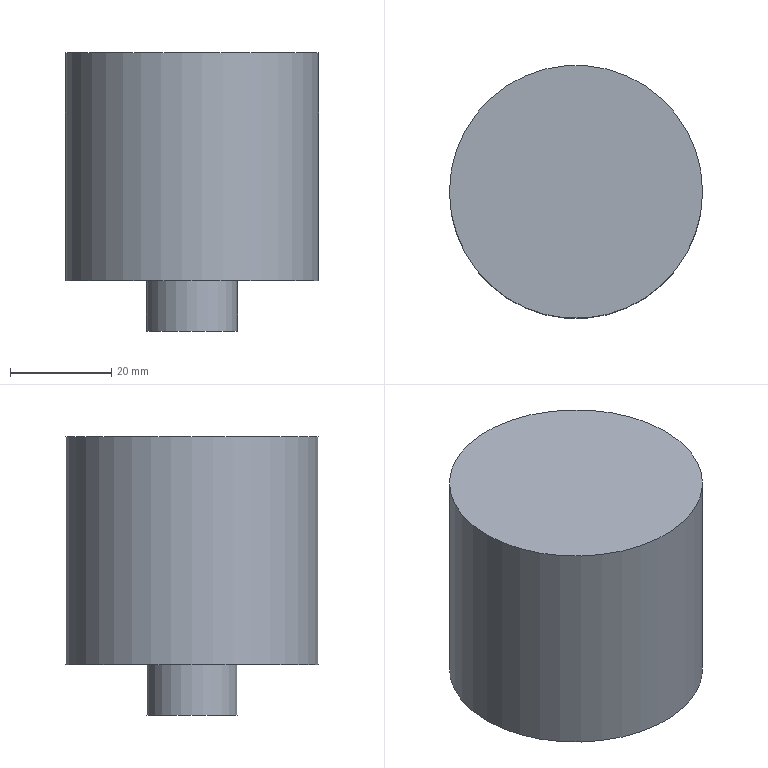Part | NX | features solid 2 | 1 solid | 5 faces | box 50 x 50 x 55 mm | volume 90902 mm3 | plane 3 | cylinder 2 | commonest cylinder face diameters 18 x1 50 x1
STEP:
#1=CARTESIAN_POINT('',(675.,-275.,-65.));
#2=VERTEX_POINT('',#1);
#3=CARTESIAN_POINT('',(650.,-275.,-65.));
#4=DIRECTION('',(0.,0.,1.));
#5=DIRECTION('',(1.,0.,0.));
#6=AXIS2_PLACEMENT_3D('',#3,#4,#5);
#7=CIRCLE('',#6,25.);
#8=EDGE_CURVE('',#2,#2,#7,.F.);
#9=ORIENTED_EDGE('',*,*,#8,.T.);
#10=EDGE_LOOP('',(#9));
#11=FACE_BOUND('',#10,.T.);
#12=CARTESIAN_POINT('',(625.,-275.,-110.));
#13=VERTEX_POINT('',#12);
#14=CARTESIAN_POINT('',(650.,-275.,-110.));
#15=DIRECTION('',(0.,0.,-1.));
#16=DIRECTION('',(-1.,0.,0.));
#17=AXIS2_PLACEMENT_3D('',#14,#15,#16);
#18=CIRCLE('',#17,25.);
#19=EDGE_CURVE('',#13,#13,#18,.T.);
#20=ORIENTED_EDGE('',*,*,#19,.F.);
#21=EDGE_LOOP('',(#20));
#22=FACE_BOUND('',#21,.T.);
#23=CARTESIAN_POINT('',(650.,-275.,-70.));
#24=DIRECTION('',(0.,0.,-1.));
#25=DIRECTION('',(1.,0.,0.));
#26=AXIS2_PLACEMENT_3D('',#23,#24,#25);
#27=CYLINDRICAL_SURFACE('',#26,25.);
#28=ADVANCED_FACE('',(#11,#22),#27,.T.);
#29=ORIENTED_EDGE('',*,*,#8,.F.);
#30=EDGE_LOOP('',(#29));
#31=FACE_BOUND('',#30,.T.);
#32=CARTESIAN_POINT('',(650.,-275.,-65.));
#33=DIRECTION('',(0.,0.,1.));
#34=DIRECTION('',(-1.,0.,0.));
#35=AXIS2_PLACEMENT_3D('',#32,#33,#34);
#36=PLANE('',#35);
#37=ADVANCED_FACE('',(#31),#36,.T.);
#38=CARTESIAN_POINT('',(641.,-275.,-110.));
#39=VERTEX_POINT('',#38);
#40=CARTESIAN_POINT('',(650.,-275.,-110.));
#41=DIRECTION('',(0.,0.,-1.));
#42=DIRECTION('',(-1.,0.,0.));
#43=AXIS2_PLACEMENT_3D('',#40,#41,#42);
#44=CIRCLE('',#43,9.);
#45=EDGE_CURVE('',#39,#39,#44,.T.);
#46=ORIENTED_EDGE('',*,*,#45,.F.);
#47=EDGE_LOOP('',(#46));
#48=FACE_BOUND('',#47,.T.);
#49=ORIENTED_EDGE('',*,*,#19,.T.);
#50=EDGE_LOOP('',(#49));
#51=FACE_BOUND('',#50,.T.);
#52=CARTESIAN_POINT('',(650.,-275.,-110.));
#53=DIRECTION('',(0.,0.,1.));
#54=DIRECTION('',(-1.,0.,0.));
#55=AXIS2_PLACEMENT_3D('',#52,#53,#54);
#56=PLANE('',#55);
#57=ADVANCED_FACE('',(#48,#51),#56,.F.);
#58=CARTESIAN_POINT('',(641.,-275.,-120.));
#59=VERTEX_POINT('',#58);
#60=CARTESIAN_POINT('',(650.,-275.,-120.));
#61=DIRECTION('',(0.,0.,-1.));
#62=DIRECTION('',(-1.,0.,0.));
#63=AXIS2_PLACEMENT_3D('',#60,#61,#62);
#64=CIRCLE('',#63,9.);
#65=EDGE_CURVE('',#59,#59,#64,.T.);
#66=ORIENTED_EDGE('',*,*,#65,.F.);
#67=EDGE_LOOP('',(#66));
#68=FACE_BOUND('',#67,.T.);
#69=ORIENTED_EDGE('',*,*,#45,.T.);
#70=EDGE_LOOP('',(#69));
#71=FACE_BOUND('',#70,.T.);
#72=CARTESIAN_POINT('',(650.,-275.,-130.));
#73=DIRECTION('',(0.,0.,1.));
#74=DIRECTION('',(-1.,0.,0.));
#75=AXIS2_PLACEMENT_3D('',#72,#73,#74);
#76=CYLINDRICAL_SURFACE('',#75,9.);
#77=ADVANCED_FACE('',(#68,#71),#76,.T.);
#78=ORIENTED_EDGE('',*,*,#65,.T.);
#79=EDGE_LOOP('',(#78));
#80=FACE_BOUND('',#79,.T.);
#81=CARTESIAN_POINT('',(650.,-275.,-120.));
#82=DIRECTION('',(0.,0.,1.));
#83=DIRECTION('',(-1.,0.,0.));
#84=AXIS2_PLACEMENT_3D('',#81,#82,#83);
#85=PLANE('',#84);
#86=ADVANCED_FACE('',(#80),#85,.F.);
#87=CLOSED_SHELL('',(#28,#37,#57,#77,#86));
#88=MANIFOLD_SOLID_BREP('',#87);
#89=(LENGTH_UNIT()NAMED_UNIT(*)SI_UNIT(.MILLI.,.METRE.));
#90=UNCERTAINTY_MEASURE_WITH_UNIT(LENGTH_MEASURE(0.00001),#89,'','');
#91=(NAMED_UNIT(*)PLANE_ANGLE_UNIT()SI_UNIT($,.RADIAN.));
#92=(NAMED_UNIT(*)SI_UNIT($,.STERADIAN.)SOLID_ANGLE_UNIT());
#93=(GEOMETRIC_REPRESENTATION_CONTEXT(3)GLOBAL_UNCERTAINTY_ASSIGNED_CONTEXT((#90))GLOBAL_UNIT_ASSIGNED_CONTEXT((#89,#91,#92))REPRESENTATION_CONTEXT('',''));
#94=ADVANCED_BREP_SHAPE_REPRESENTATION('',(#88),#93);